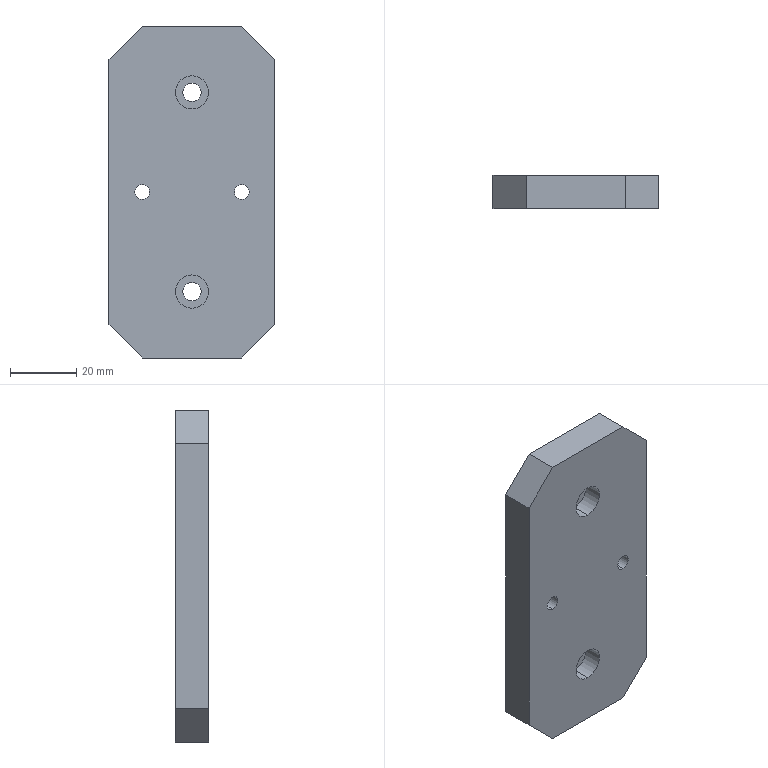Part | STEP file | PN_0019 | 1 solid | 54 faces | box 50 x 10 x 100 mm | volume 45504 mm3 | cylinder 28 | plane 14 | cone 12 | commonest cylinder face diameters 4 x8 3.3 x4 4.5 x4 5.5 x4 8 x4 10 x4